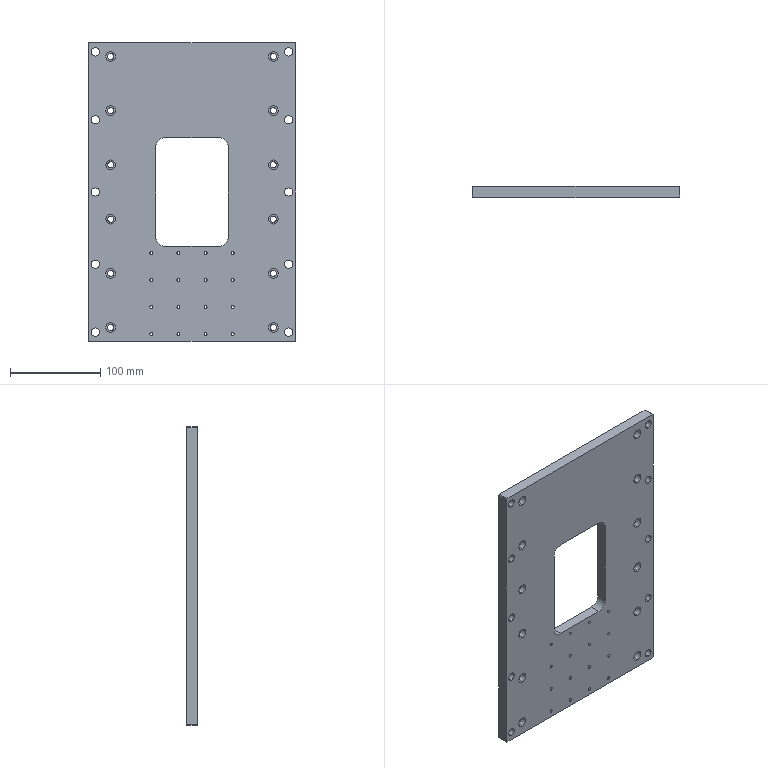Part | SolidWorks | features HoleWzd 3, Chamfer 1, Extrusion 1, Fillet 1, ICE 1 | 1 solid | 130 faces | box 230 x 12 x 330 mm | volume 777440 mm3 | cylinder 104 | plane 26 | commonest cylinder face diameters 3.3 x32 6.6 x24 11 x24 9 x20 20 x4